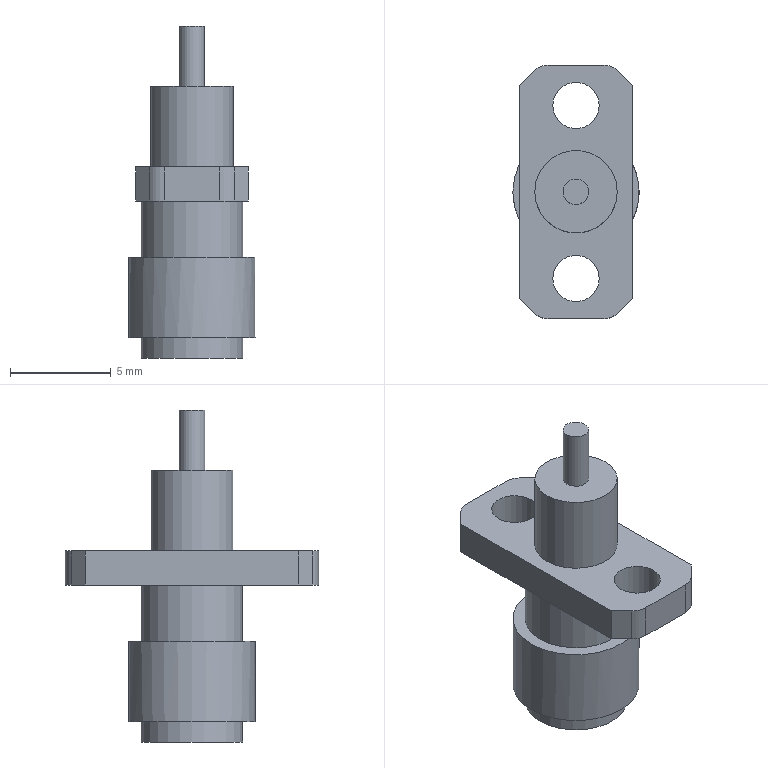Part | STEP file | SMA-KFD-4-3 | 1 solid | 26 faces | box 6.28 x 12.6 x 16.5 mm | volume 359.204 mm3 | plane 15 | cylinder 11 | commonest cylinder face diameters 2 x4 2.3 x2 5.06 x2 1.27 x1 4.1 x1 6.28 x1